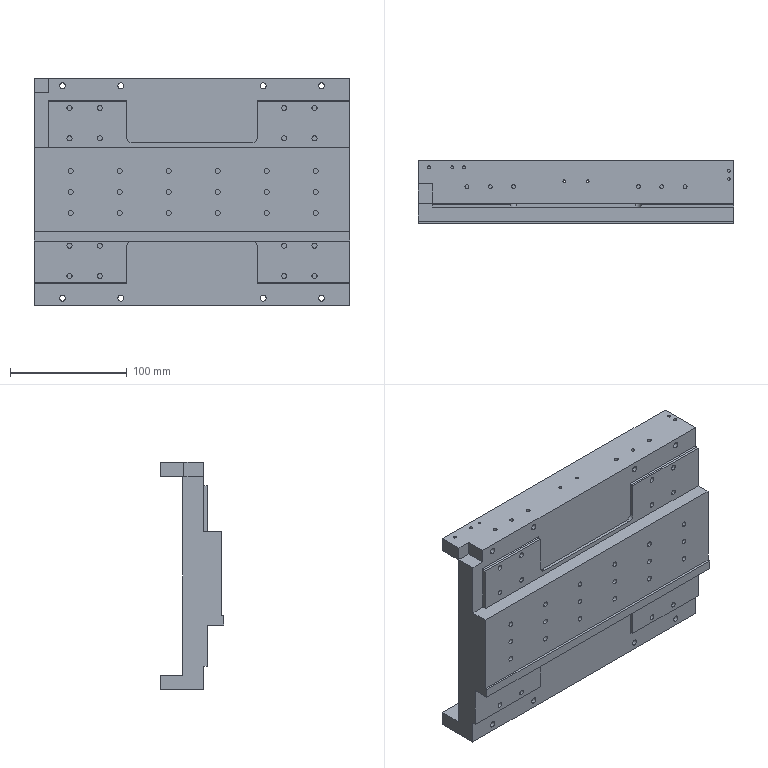Part | SolidWorks | features BaseBody 1 | 1 solid | 272 faces | box 270 x 54 x 195 mm | volume 1409975 mm3 | cylinder 173 | plane 91 | cone 8 | commonest cylinder face diameters 4.5 x68 8 x36 5 x24 2.5 x21 3.3 x12 10 x8